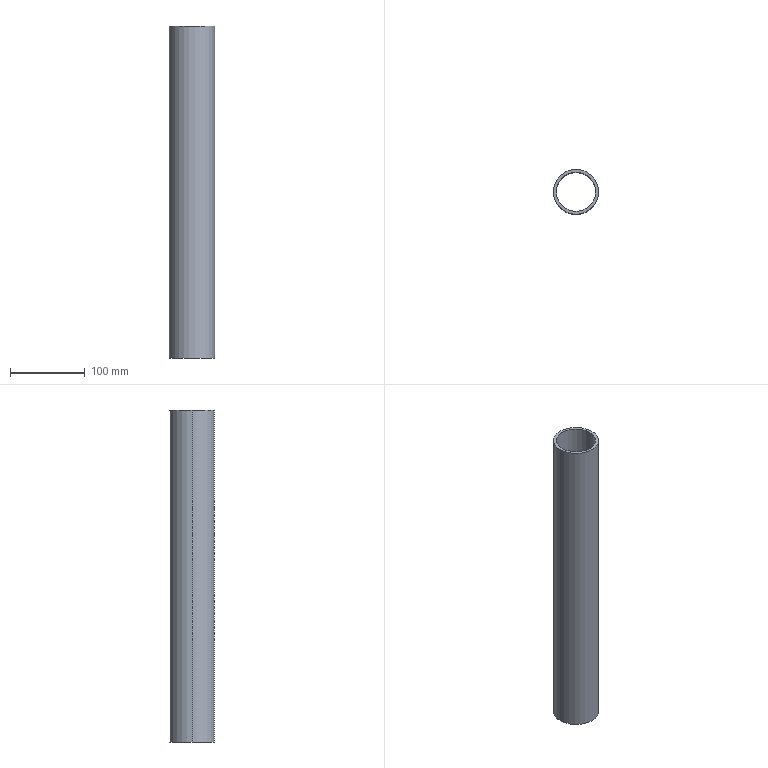Part | SolidWorks | features Extrusion 1 | 1 solid | 6 faces | box 60.325 x 60.325 x 444.5 mm | volume 308147 mm3 | cylinder 4 | plane 2 | commonest cylinder face diameters 52.502 x2 60.325 x2
STEP:
#1=CARTESIAN_POINT('',(-26.251,0.,222.25));
#2=VERTEX_POINT('',#1);
#3=CARTESIAN_POINT('',(26.251,0.,222.25));
#4=VERTEX_POINT('',#3);
#5=CARTESIAN_POINT('',(0.,0.,222.25));
#6=DIRECTION('',(0.,0.,1.));
#7=DIRECTION('',(1.,0.,0.));
#8=AXIS2_PLACEMENT_3D('',#5,#6,#7);
#9=CIRCLE('',#8,26.251);
#10=EDGE_CURVE('',#2,#4,#9,.T.);
#11=ORIENTED_EDGE('',*,*,#10,.T.);
#12=CARTESIAN_POINT('',(26.251,0.,-222.25));
#13=VERTEX_POINT('',#12);
#14=CARTESIAN_POINT('',(26.251,0.,222.25));
#15=DIRECTION('',(0.,0.,-1.));
#16=VECTOR('',#15,1000.);
#17=LINE('',#14,#16);
#18=EDGE_CURVE('',#4,#13,#17,.T.);
#19=ORIENTED_EDGE('',*,*,#18,.T.);
#20=CARTESIAN_POINT('',(-26.251,0.,-222.25));
#21=VERTEX_POINT('',#20);
#22=CARTESIAN_POINT('',(0.,0.,-222.25));
#23=DIRECTION('',(0.,0.,1.));
#24=DIRECTION('',(1.,0.,0.));
#25=AXIS2_PLACEMENT_3D('',#22,#23,#24);
#26=CIRCLE('',#25,26.251);
#27=EDGE_CURVE('',#21,#13,#26,.T.);
#28=ORIENTED_EDGE('',*,*,#27,.F.);
#29=CARTESIAN_POINT('',(-26.251,0.,222.25));
#30=DIRECTION('',(0.,0.,-1.));
#31=VECTOR('',#30,1000.);
#32=LINE('',#29,#31);
#33=EDGE_CURVE('',#2,#21,#32,.T.);
#34=ORIENTED_EDGE('',*,*,#33,.F.);
#35=EDGE_LOOP('',(#11,#19,#28,#34));
#36=FACE_OUTER_BOUND('',#35,.T.);
#37=CARTESIAN_POINT('',(0.,0.,222.25));
#38=DIRECTION('',(0.,0.,-1.));
#39=DIRECTION('',(-1.,0.,0.));
#40=AXIS2_PLACEMENT_3D('',#37,#38,#39);
#41=CYLINDRICAL_SURFACE('',#40,26.251);
#42=ADVANCED_FACE('',(#36),#41,.F.);
#43=CARTESIAN_POINT('',(30.162,0.,222.25));
#44=VERTEX_POINT('',#43);
#45=CARTESIAN_POINT('',(-30.162,0.,222.25));
#46=VERTEX_POINT('',#45);
#47=CARTESIAN_POINT('',(0.,0.,222.25));
#48=DIRECTION('',(0.,0.,1.));
#49=DIRECTION('',(1.,0.,0.));
#50=AXIS2_PLACEMENT_3D('',#47,#48,#49);
#51=CIRCLE('',#50,30.162);
#52=EDGE_CURVE('',#44,#46,#51,.T.);
#53=ORIENTED_EDGE('',*,*,#52,.F.);
#54=CARTESIAN_POINT('',(30.162,0.,-222.25));
#55=VERTEX_POINT('',#54);
#56=CARTESIAN_POINT('',(30.162,0.,222.25));
#57=DIRECTION('',(0.,0.,-1.));
#58=VECTOR('',#57,1000.);
#59=LINE('',#56,#58);
#60=EDGE_CURVE('',#44,#55,#59,.T.);
#61=ORIENTED_EDGE('',*,*,#60,.T.);
#62=CARTESIAN_POINT('',(-30.162,0.,-222.25));
#63=VERTEX_POINT('',#62);
#64=CARTESIAN_POINT('',(0.,0.,-222.25));
#65=DIRECTION('',(0.,0.,1.));
#66=DIRECTION('',(1.,0.,0.));
#67=AXIS2_PLACEMENT_3D('',#64,#65,#66);
#68=CIRCLE('',#67,30.162);
#69=EDGE_CURVE('',#55,#63,#68,.T.);
#70=ORIENTED_EDGE('',*,*,#69,.T.);
#71=CARTESIAN_POINT('',(-30.162,0.,222.25));
#72=DIRECTION('',(0.,0.,-1.));
#73=VECTOR('',#72,1000.);
#74=LINE('',#71,#73);
#75=EDGE_CURVE('',#46,#63,#74,.T.);
#76=ORIENTED_EDGE('',*,*,#75,.F.);
#77=EDGE_LOOP('',(#53,#61,#70,#76));
#78=FACE_OUTER_BOUND('',#77,.T.);
#79=CARTESIAN_POINT('',(0.,0.,222.25));
#80=DIRECTION('',(0.,0.,-1.));
#81=DIRECTION('',(-1.,0.,0.));
#82=AXIS2_PLACEMENT_3D('',#79,#80,#81);
#83=CYLINDRICAL_SURFACE('',#82,30.162);
#84=ADVANCED_FACE('',(#78),#83,.T.);
#85=CARTESIAN_POINT('',(0.,0.,222.25));
#86=DIRECTION('',(0.,0.,1.));
#87=DIRECTION('',(1.,0.,0.));
#88=AXIS2_PLACEMENT_3D('',#85,#86,#87);
#89=CIRCLE('',#88,30.162);
#90=EDGE_CURVE('',#46,#44,#89,.T.);
#91=ORIENTED_EDGE('',*,*,#90,.T.);
#92=ORIENTED_EDGE('',*,*,#52,.T.);
#93=EDGE_LOOP('',(#91,#92));
#94=FACE_OUTER_BOUND('',#93,.T.);
#95=ORIENTED_EDGE('',*,*,#10,.F.);
#96=CARTESIAN_POINT('',(0.,0.,222.25));
#97=DIRECTION('',(0.,0.,1.));
#98=DIRECTION('',(1.,0.,0.));
#99=AXIS2_PLACEMENT_3D('',#96,#97,#98);
#100=CIRCLE('',#99,26.251);
#101=EDGE_CURVE('',#4,#2,#100,.T.);
#102=ORIENTED_EDGE('',*,*,#101,.F.);
#103=EDGE_LOOP('',(#95,#102));
#104=FACE_BOUND('',#103,.T.);
#105=CARTESIAN_POINT('',(0.,0.,222.25));
#106=DIRECTION('',(0.,0.,1.));
#107=DIRECTION('',(1.,0.,0.));
#108=AXIS2_PLACEMENT_3D('',#105,#106,#107);
#109=PLANE('',#108);
#110=ADVANCED_FACE('',(#94,#104),#109,.T.);
#111=ORIENTED_EDGE('',*,*,#60,.F.);
#112=ORIENTED_EDGE('',*,*,#90,.F.);
#113=ORIENTED_EDGE('',*,*,#75,.T.);
#114=CARTESIAN_POINT('',(0.,0.,-222.25));
#115=DIRECTION('',(0.,0.,1.));
#116=DIRECTION('',(1.,0.,0.));
#117=AXIS2_PLACEMENT_3D('',#114,#115,#116);
#118=CIRCLE('',#117,30.162);
#119=EDGE_CURVE('',#63,#55,#118,.T.);
#120=ORIENTED_EDGE('',*,*,#119,.T.);
#121=EDGE_LOOP('',(#111,#112,#113,#120));
#122=FACE_OUTER_BOUND('',#121,.T.);
#123=CARTESIAN_POINT('',(0.,0.,222.25));
#124=DIRECTION('',(0.,0.,-1.));
#125=DIRECTION('',(-1.,0.,0.));
#126=AXIS2_PLACEMENT_3D('',#123,#124,#125);
#127=CYLINDRICAL_SURFACE('',#126,30.162);
#128=ADVANCED_FACE('',(#122),#127,.T.);
#129=ORIENTED_EDGE('',*,*,#18,.F.);
#130=ORIENTED_EDGE('',*,*,#101,.T.);
#131=ORIENTED_EDGE('',*,*,#33,.T.);
#132=CARTESIAN_POINT('',(0.,0.,-222.25));
#133=DIRECTION('',(0.,0.,1.));
#134=DIRECTION('',(1.,0.,0.));
#135=AXIS2_PLACEMENT_3D('',#132,#133,#134);
#136=CIRCLE('',#135,26.251);
#137=EDGE_CURVE('',#13,#21,#136,.T.);
#138=ORIENTED_EDGE('',*,*,#137,.F.);
#139=EDGE_LOOP('',(#129,#130,#131,#138));
#140=FACE_OUTER_BOUND('',#139,.T.);
#141=CARTESIAN_POINT('',(0.,0.,222.25));
#142=DIRECTION('',(0.,0.,-1.));
#143=DIRECTION('',(-1.,0.,0.));
#144=AXIS2_PLACEMENT_3D('',#141,#142,#143);
#145=CYLINDRICAL_SURFACE('',#144,26.251);
#146=ADVANCED_FACE('',(#140),#145,.F.);
#147=ORIENTED_EDGE('',*,*,#27,.T.);
#148=ORIENTED_EDGE('',*,*,#137,.T.);
#149=EDGE_LOOP('',(#147,#148));
#150=FACE_BOUND('',#149,.T.);
#151=ORIENTED_EDGE('',*,*,#119,.F.);
#152=ORIENTED_EDGE('',*,*,#69,.F.);
#153=EDGE_LOOP('',(#151,#152));
#154=FACE_OUTER_BOUND('',#153,.T.);
#155=CARTESIAN_POINT('',(0.,0.,-222.25));
#156=DIRECTION('',(0.,0.,1.));
#157=DIRECTION('',(1.,0.,0.));
#158=AXIS2_PLACEMENT_3D('',#155,#156,#157);
#159=PLANE('',#158);
#160=ADVANCED_FACE('',(#150,#154),#159,.F.);
#161=CLOSED_SHELL('',(#42,#84,#110,#128,#146,#160));
#162=MANIFOLD_SOLID_BREP('',#161);
#163=CARTESIAN_POINT('',(0.,0.,0.));
#164=DIRECTION('',(0.,0.,1.));
#165=DIRECTION('',(1.,0.,0.));
#166=AXIS2_PLACEMENT_3D('',#163,#164,#165);
#167=(LENGTH_UNIT()NAMED_UNIT(*)SI_UNIT(.MILLI.,.METRE.));
#168=UNCERTAINTY_MEASURE_WITH_UNIT(LENGTH_MEASURE(0.00001),#167,'','');
#169=(NAMED_UNIT(*)PLANE_ANGLE_UNIT()SI_UNIT($,.RADIAN.));
#170=(NAMED_UNIT(*)SI_UNIT($,.STERADIAN.)SOLID_ANGLE_UNIT());
#171=(GEOMETRIC_REPRESENTATION_CONTEXT(3)GLOBAL_UNCERTAINTY_ASSIGNED_CONTEXT((#168))GLOBAL_UNIT_ASSIGNED_CONTEXT((#167,#169,#170))REPRESENTATION_CONTEXT('',''));
#172=ADVANCED_BREP_SHAPE_REPRESENTATION('',(#162,#166),#171);